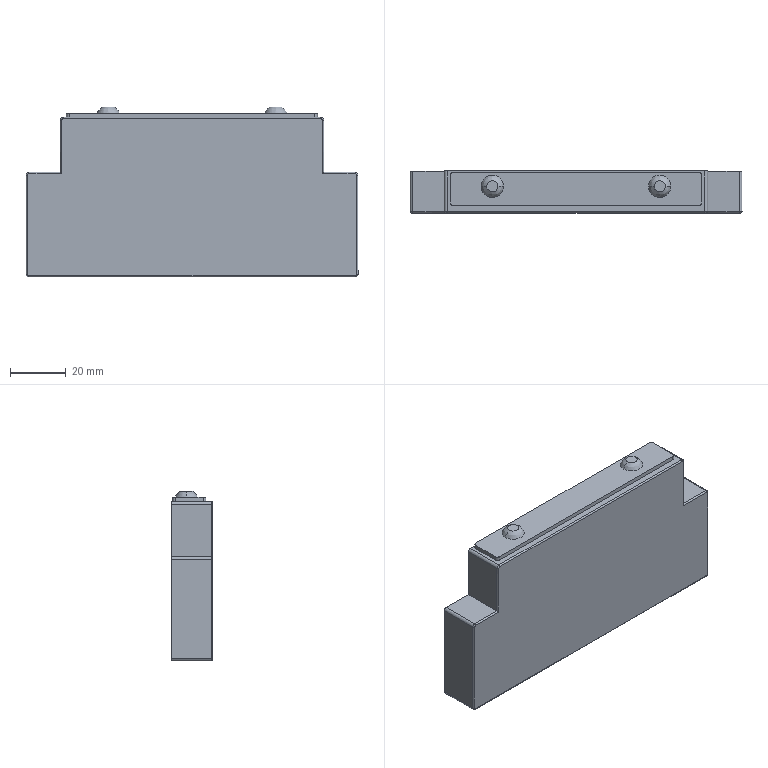Part | SolidWorks | features BaseBody 1 | 1 solid | 45 faces | box 119 x 15 x 60.9 mm | volume 96566 mm3 | cylinder 18 | plane 17 | spline 10 | commonest cylinder face diameters 2 x10 1 x8